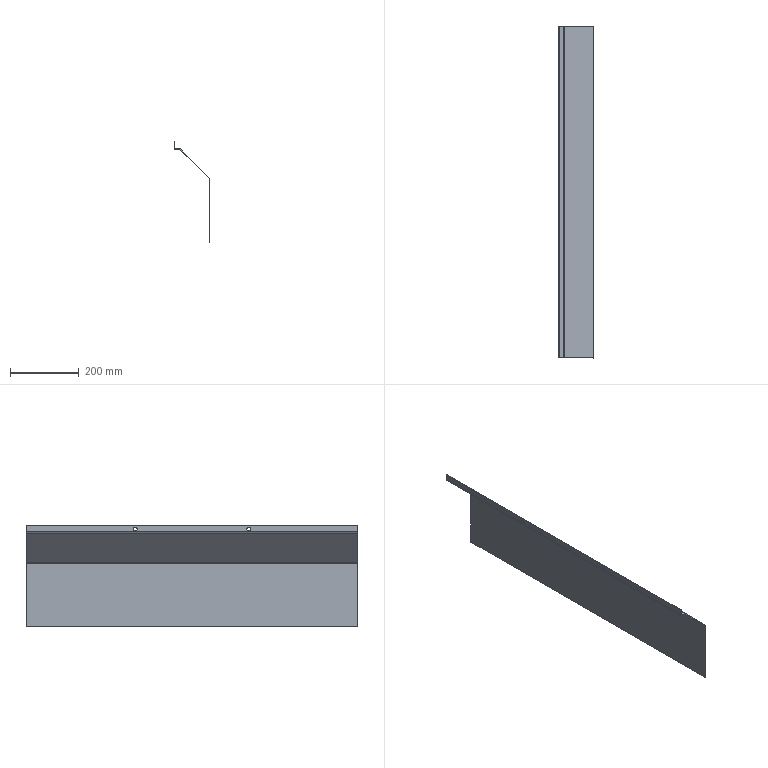Part | STEP file | SYL_0392D6J1SYL0380DJ100-474592 | 1 solid | 38 faces | box 104 x 964 x 292 mm | volume 494830 mm3 | plane 28 | cylinder 10 | commonest cylinder face diameters 8 x4 4 x3 7 x3
STEP:
#1=CARTESIAN_POINT('',(0.,163.,6.));
#2=VERTEX_POINT('',#1);
#3=CARTESIAN_POINT('',(-1.5,163.,6.));
#4=VERTEX_POINT('',#3);
#5=CARTESIAN_POINT('',(-1.5,163.,6.));
#6=DIRECTION('',(-1.,0.,0.));
#7=VECTOR('',#6,1000.);
#8=LINE('',#5,#7);
#9=EDGE_CURVE('',#2,#4,#8,.T.);
#10=ORIENTED_EDGE('',*,*,#9,.F.);
#11=CARTESIAN_POINT('',(0.,167.,6.));
#12=VERTEX_POINT('',#11);
#13=CARTESIAN_POINT('',(0.,-482.,6.));
#14=DIRECTION('',(0.,1.,0.));
#15=VECTOR('',#14,1000.);
#16=LINE('',#13,#15);
#17=EDGE_CURVE('',#2,#12,#16,.T.);
#18=ORIENTED_EDGE('',*,*,#17,.T.);
#19=CARTESIAN_POINT('',(-1.5,167.,6.));
#20=VERTEX_POINT('',#19);
#21=CARTESIAN_POINT('',(-1.5,167.,6.));
#22=DIRECTION('',(-1.,0.,0.));
#23=VECTOR('',#22,1000.);
#24=LINE('',#21,#23);
#25=EDGE_CURVE('',#12,#20,#24,.T.);
#26=ORIENTED_EDGE('',*,*,#25,.T.);
#27=CARTESIAN_POINT('',(-1.5,163.,6.));
#28=DIRECTION('',(0.,1.,0.));
#29=VECTOR('',#28,1000.);
#30=LINE('',#27,#29);
#31=EDGE_CURVE('',#4,#20,#30,.T.);
#32=ORIENTED_EDGE('',*,*,#31,.F.);
#33=EDGE_LOOP('',(#10,#18,#26,#32));
#34=FACE_OUTER_BOUND('',#33,.T.);
#35=CARTESIAN_POINT('',(-1.5,163.,6.));
#36=DIRECTION('',(0.,0.,-1.));
#37=DIRECTION('',(0.,1.,0.));
#38=AXIS2_PLACEMENT_3D('',#35,#36,#37);
#39=PLANE('',#38);
#40=ADVANCED_FACE('',(#34),#39,.F.);
#41=ORIENTED_EDGE('',*,*,#25,.F.);
#42=CARTESIAN_POINT('',(0.,167.,14.));
#43=VERTEX_POINT('',#42);
#44=CARTESIAN_POINT('',(0.,167.,10.));
#45=DIRECTION('',(1.,0.,0.));
#46=DIRECTION('',(0.,0.,-1.));
#47=AXIS2_PLACEMENT_3D('',#44,#45,#46);
#48=CIRCLE('',#47,4.);
#49=EDGE_CURVE('',#12,#43,#48,.T.);
#50=ORIENTED_EDGE('',*,*,#49,.T.);
#51=CARTESIAN_POINT('',(-1.5,167.,14.));
#52=VERTEX_POINT('',#51);
#53=CARTESIAN_POINT('',(-1.5,167.,14.));
#54=DIRECTION('',(-1.,0.,0.));
#55=VECTOR('',#54,1000.);
#56=LINE('',#53,#55);
#57=EDGE_CURVE('',#43,#52,#56,.T.);
#58=ORIENTED_EDGE('',*,*,#57,.T.);
#59=CARTESIAN_POINT('',(-1.5,167.,10.));
#60=DIRECTION('',(1.,0.,0.));
#61=DIRECTION('',(0.,0.,-1.));
#62=AXIS2_PLACEMENT_3D('',#59,#60,#61);
#63=CIRCLE('',#62,4.);
#64=EDGE_CURVE('',#20,#52,#63,.T.);
#65=ORIENTED_EDGE('',*,*,#64,.F.);
#66=EDGE_LOOP('',(#41,#50,#58,#65));
#67=FACE_OUTER_BOUND('',#66,.T.);
#68=CARTESIAN_POINT('',(-1.5,167.,10.));
#69=DIRECTION('',(1.,0.,0.));
#70=DIRECTION('',(0.,0.,-1.));
#71=AXIS2_PLACEMENT_3D('',#68,#69,#70);
#72=CYLINDRICAL_SURFACE('',#71,4.);
#73=ADVANCED_FACE('',(#67),#72,.F.);
#74=ORIENTED_EDGE('',*,*,#57,.F.);
#75=CARTESIAN_POINT('',(0.,163.,14.));
#76=VERTEX_POINT('',#75);
#77=CARTESIAN_POINT('',(0.,-482.,14.));
#78=DIRECTION('',(0.,-1.,0.));
#79=VECTOR('',#78,1000.);
#80=LINE('',#77,#79);
#81=EDGE_CURVE('',#43,#76,#80,.T.);
#82=ORIENTED_EDGE('',*,*,#81,.T.);
#83=CARTESIAN_POINT('',(-1.5,163.,14.));
#84=VERTEX_POINT('',#83);
#85=CARTESIAN_POINT('',(-1.5,163.,14.));
#86=DIRECTION('',(-1.,0.,0.));
#87=VECTOR('',#86,1000.);
#88=LINE('',#85,#87);
#89=EDGE_CURVE('',#76,#84,#88,.T.);
#90=ORIENTED_EDGE('',*,*,#89,.T.);
#91=CARTESIAN_POINT('',(-1.5,167.,14.));
#92=DIRECTION('',(0.,-1.,0.));
#93=VECTOR('',#92,1000.);
#94=LINE('',#91,#93);
#95=EDGE_CURVE('',#52,#84,#94,.T.);
#96=ORIENTED_EDGE('',*,*,#95,.F.);
#97=EDGE_LOOP('',(#74,#82,#90,#96));
#98=FACE_OUTER_BOUND('',#97,.T.);
#99=CARTESIAN_POINT('',(-1.5,167.,14.));
#100=DIRECTION('',(0.,0.,1.));
#101=DIRECTION('',(0.,-1.,0.));
#102=AXIS2_PLACEMENT_3D('',#99,#100,#101);
#103=PLANE('',#102);
#104=ADVANCED_FACE('',(#98),#103,.F.);
#105=CARTESIAN_POINT('',(0.,-163.,6.));
#106=VERTEX_POINT('',#105);
#107=CARTESIAN_POINT('',(-1.5,-163.,6.));
#108=VERTEX_POINT('',#107);
#109=CARTESIAN_POINT('',(-1.5,-163.,6.));
#110=DIRECTION('',(-1.,0.,0.));
#111=VECTOR('',#110,1000.);
#112=LINE('',#109,#111);
#113=EDGE_CURVE('',#106,#108,#112,.T.);
#114=ORIENTED_EDGE('',*,*,#113,.F.);
#115=CARTESIAN_POINT('',(0.,-163.,14.));
#116=VERTEX_POINT('',#115);
#117=CARTESIAN_POINT('',(0.,-163.,10.));
#118=DIRECTION('',(1.,0.,0.));
#119=DIRECTION('',(0.,0.,-1.));
#120=AXIS2_PLACEMENT_3D('',#117,#118,#119);
#121=CIRCLE('',#120,4.);
#122=EDGE_CURVE('',#106,#116,#121,.T.);
#123=ORIENTED_EDGE('',*,*,#122,.T.);
#124=CARTESIAN_POINT('',(-1.5,-163.,14.));
#125=VERTEX_POINT('',#124);
#126=CARTESIAN_POINT('',(-1.5,-163.,14.));
#127=DIRECTION('',(-1.,0.,0.));
#128=VECTOR('',#127,1000.);
#129=LINE('',#126,#128);
#130=EDGE_CURVE('',#116,#125,#129,.T.);
#131=ORIENTED_EDGE('',*,*,#130,.T.);
#132=CARTESIAN_POINT('',(-1.5,-163.,10.));
#133=DIRECTION('',(1.,0.,0.));
#134=DIRECTION('',(0.,0.,-1.));
#135=AXIS2_PLACEMENT_3D('',#132,#133,#134);
#136=CIRCLE('',#135,4.);
#137=EDGE_CURVE('',#108,#125,#136,.T.);
#138=ORIENTED_EDGE('',*,*,#137,.F.);
#139=EDGE_LOOP('',(#114,#123,#131,#138));
#140=FACE_OUTER_BOUND('',#139,.T.);
#141=CARTESIAN_POINT('',(-1.5,-163.,10.));
#142=DIRECTION('',(1.,0.,0.));
#143=DIRECTION('',(0.,0.,-1.));
#144=AXIS2_PLACEMENT_3D('',#141,#142,#143);
#145=CYLINDRICAL_SURFACE('',#144,4.);
#146=ADVANCED_FACE('',(#140),#145,.F.);
#147=ORIENTED_EDGE('',*,*,#130,.F.);
#148=CARTESIAN_POINT('',(0.,-167.,14.));
#149=VERTEX_POINT('',#148);
#150=CARTESIAN_POINT('',(0.,-482.,14.));
#151=DIRECTION('',(0.,-1.,0.));
#152=VECTOR('',#151,1000.);
#153=LINE('',#150,#152);
#154=EDGE_CURVE('',#116,#149,#153,.T.);
#155=ORIENTED_EDGE('',*,*,#154,.T.);
#156=CARTESIAN_POINT('',(-1.5,-167.,14.));
#157=VERTEX_POINT('',#156);
#158=CARTESIAN_POINT('',(-1.5,-167.,14.));
#159=DIRECTION('',(-1.,0.,0.));
#160=VECTOR('',#159,1000.);
#161=LINE('',#158,#160);
#162=EDGE_CURVE('',#149,#157,#161,.T.);
#163=ORIENTED_EDGE('',*,*,#162,.T.);
#164=CARTESIAN_POINT('',(-1.5,-163.,14.));
#165=DIRECTION('',(0.,-1.,0.));
#166=VECTOR('',#165,1000.);
#167=LINE('',#164,#166);
#168=EDGE_CURVE('',#125,#157,#167,.T.);
#169=ORIENTED_EDGE('',*,*,#168,.F.);
#170=EDGE_LOOP('',(#147,#155,#163,#169));
#171=FACE_OUTER_BOUND('',#170,.T.);
#172=CARTESIAN_POINT('',(-1.5,-163.,14.));
#173=DIRECTION('',(0.,0.,1.));
#174=DIRECTION('',(0.,-1.,0.));
#175=AXIS2_PLACEMENT_3D('',#172,#173,#174);
#176=PLANE('',#175);
#177=ADVANCED_FACE('',(#171),#176,.F.);
#178=ORIENTED_EDGE('',*,*,#162,.F.);
#179=CARTESIAN_POINT('',(0.,-167.,6.));
#180=VERTEX_POINT('',#179);
#181=CARTESIAN_POINT('',(0.,-167.,10.));
#182=DIRECTION('',(1.,0.,0.));
#183=DIRECTION('',(0.,0.,-1.));
#184=AXIS2_PLACEMENT_3D('',#181,#182,#183);
#185=CIRCLE('',#184,4.);
#186=EDGE_CURVE('',#149,#180,#185,.T.);
#187=ORIENTED_EDGE('',*,*,#186,.T.);
#188=CARTESIAN_POINT('',(-1.5,-167.,6.));
#189=VERTEX_POINT('',#188);
#190=CARTESIAN_POINT('',(-1.5,-167.,6.));
#191=DIRECTION('',(-1.,0.,0.));
#192=VECTOR('',#191,1000.);
#193=LINE('',#190,#192);
#194=EDGE_CURVE('',#180,#189,#193,.T.);
#195=ORIENTED_EDGE('',*,*,#194,.T.);
#196=CARTESIAN_POINT('',(-1.5,-167.,10.));
#197=DIRECTION('',(1.,0.,0.));
#198=DIRECTION('',(0.,0.,1.));
#199=AXIS2_PLACEMENT_3D('',#196,#197,#198);
#200=CIRCLE('',#199,4.);
#201=EDGE_CURVE('',#157,#189,#200,.T.);
#202=ORIENTED_EDGE('',*,*,#201,.F.);
#203=EDGE_LOOP('',(#178,#187,#195,#202));
#204=FACE_OUTER_BOUND('',#203,.T.);
#205=CARTESIAN_POINT('',(-1.5,-167.,10.));
#206=DIRECTION('',(1.,0.,0.));
#207=DIRECTION('',(0.,0.,-1.));
#208=AXIS2_PLACEMENT_3D('',#205,#206,#207);
#209=CYLINDRICAL_SURFACE('',#208,4.);
#210=ADVANCED_FACE('',(#204),#209,.F.);
#211=CARTESIAN_POINT('',(0.,-482.,20.));
#212=VERTEX_POINT('',#211);
#213=CARTESIAN_POINT('',(-1.5,-482.,20.));
#214=VERTEX_POINT('',#213);
#215=CARTESIAN_POINT('',(-1.5,-482.,20.));
#216=DIRECTION('',(-1.,0.,0.));
#217=VECTOR('',#216,1000.);
#218=LINE('',#215,#217);
#219=EDGE_CURVE('',#212,#214,#218,.T.);
#220=ORIENTED_EDGE('',*,*,#219,.F.);
#221=CARTESIAN_POINT('',(0.,482.,20.));
#222=VERTEX_POINT('',#221);
#223=CARTESIAN_POINT('',(0.,-482.,20.));
#224=DIRECTION('',(0.,-1.,0.));
#225=VECTOR('',#224,1000.);
#226=LINE('',#223,#225);
#227=EDGE_CURVE('',#222,#212,#226,.T.);
#228=ORIENTED_EDGE('',*,*,#227,.F.);
#229=CARTESIAN_POINT('',(-1.5,482.,20.));
#230=VERTEX_POINT('',#229);
#231=CARTESIAN_POINT('',(-1.5,482.,20.));
#232=DIRECTION('',(-1.,0.,0.));
#233=VECTOR('',#232,1000.);
#234=LINE('',#231,#233);
#235=EDGE_CURVE('',#222,#230,#234,.T.);
#236=ORIENTED_EDGE('',*,*,#235,.T.);
#237=CARTESIAN_POINT('',(-1.5,482.,20.));
#238=DIRECTION('',(0.,-1.,0.));
#239=VECTOR('',#238,1000.);
#240=LINE('',#237,#239);
#241=EDGE_CURVE('',#230,#214,#240,.T.);
#242=ORIENTED_EDGE('',*,*,#241,.T.);
#243=EDGE_LOOP('',(#220,#228,#236,#242));
#244=FACE_OUTER_BOUND('',#243,.T.);
#245=CARTESIAN_POINT('',(-1.5,482.,20.));
#246=DIRECTION('',(0.,0.,1.));
#247=DIRECTION('',(0.,-1.,0.));
#248=AXIS2_PLACEMENT_3D('',#245,#246,#247);
#249=PLANE('',#248);
#250=ADVANCED_FACE('',(#244),#249,.T.);
#251=ORIENTED_EDGE('',*,*,#235,.F.);
#252=CARTESIAN_POINT('',(0.,482.,2.));
#253=VERTEX_POINT('',#252);
#254=CARTESIAN_POINT('',(0.,482.,20.));
#255=DIRECTION('',(0.,0.,1.));
#256=VECTOR('',#255,1000.);
#257=LINE('',#254,#256);
#258=EDGE_CURVE('',#253,#222,#257,.T.);
#259=ORIENTED_EDGE('',*,*,#258,.F.);
#260=CARTESIAN_POINT('',(-1.5,482.,2.));
#261=VERTEX_POINT('',#260);
#262=CARTESIAN_POINT('',(-1.5,482.,2.));
#263=DIRECTION('',(-1.,0.,0.));
#264=VECTOR('',#263,1000.);
#265=LINE('',#262,#264);
#266=EDGE_CURVE('',#253,#261,#265,.T.);
#267=ORIENTED_EDGE('',*,*,#266,.T.);
#268=CARTESIAN_POINT('',(-1.5,482.,2.));
#269=DIRECTION('',(0.,0.,1.));
#270=VECTOR('',#269,1000.);
#271=LINE('',#268,#270);
#272=EDGE_CURVE('',#261,#230,#271,.T.);
#273=ORIENTED_EDGE('',*,*,#272,.T.);
#274=EDGE_LOOP('',(#251,#259,#267,#273));
#275=FACE_OUTER_BOUND('',#274,.T.);
#276=CARTESIAN_POINT('',(-1.5,482.,2.));
#277=DIRECTION('',(0.,1.,0.));
#278=DIRECTION('',(0.,0.,1.));
#279=AXIS2_PLACEMENT_3D('',#276,#277,#278);
#280=PLANE('',#279);
#281=ADVANCED_FACE('',(#275),#280,.T.);
#282=ORIENTED_EDGE('',*,*,#266,.F.);
#283=CARTESIAN_POINT('',(2.,482.,0.));
#284=VERTEX_POINT('',#283);
#285=CARTESIAN_POINT('',(2.,482.,2.));
#286=DIRECTION('',(0.,1.,0.));
#287=DIRECTION('',(0.,0.,1.));
#288=AXIS2_PLACEMENT_3D('',#285,#286,#287);
#289=CIRCLE('',#288,2.);
#290=EDGE_CURVE('',#284,#253,#289,.T.);
#291=ORIENTED_EDGE('',*,*,#290,.F.);
#292=CARTESIAN_POINT('',(2.,482.,-1.5));
#293=VERTEX_POINT('',#292);
#294=CARTESIAN_POINT('',(2.,482.,-1.5));
#295=DIRECTION('',(0.,0.,-1.));
#296=VECTOR('',#295,1000.);
#297=LINE('',#294,#296);
#298=EDGE_CURVE('',#284,#293,#297,.T.);
#299=ORIENTED_EDGE('',*,*,#298,.T.);
#300=CARTESIAN_POINT('',(2.,482.,2.));
#301=DIRECTION('',(0.,1.,0.));
#302=DIRECTION('',(0.,0.,-1.));
#303=AXIS2_PLACEMENT_3D('',#300,#301,#302);
#304=CIRCLE('',#303,3.5);
#305=EDGE_CURVE('',#293,#261,#304,.T.);
#306=ORIENTED_EDGE('',*,*,#305,.T.);
#307=EDGE_LOOP('',(#282,#291,#299,#306));
#308=FACE_OUTER_BOUND('',#307,.T.);
#309=CARTESIAN_POINT('',(2.,482.,2.));
#310=DIRECTION('',(0.,-1.,0.));
#311=DIRECTION('',(0.,0.,-1.));
#312=AXIS2_PLACEMENT_3D('',#309,#310,#311);
#313=PLANE('',#312);
#314=ADVANCED_FACE('',(#308),#313,.F.);
#315=ORIENTED_EDGE('',*,*,#298,.F.);
#316=CARTESIAN_POINT('',(14.05,482.,0.));
#317=VERTEX_POINT('',#316);
#318=CARTESIAN_POINT('',(0.,482.,0.));
#319=DIRECTION('',(-1.,0.,0.));
#320=VECTOR('',#319,1000.);
#321=LINE('',#318,#320);
#322=EDGE_CURVE('',#317,#284,#321,.T.);
#323=ORIENTED_EDGE('',*,*,#322,.F.);
#324=CARTESIAN_POINT('',(14.05,482.,-1.5));
#325=VERTEX_POINT('',#324);
#326=CARTESIAN_POINT('',(14.05,482.,-1.5));
#327=DIRECTION('',(0.,0.,-1.));
#328=VECTOR('',#327,1000.);
#329=LINE('',#326,#328);
#330=EDGE_CURVE('',#317,#325,#329,.T.);
#331=ORIENTED_EDGE('',*,*,#330,.T.);
#332=CARTESIAN_POINT('',(14.05,482.,-1.5));
#333=DIRECTION('',(-1.,0.,0.));
#334=VECTOR('',#333,1000.);
#335=LINE('',#332,#334);
#336=EDGE_CURVE('',#325,#293,#335,.T.);
#337=ORIENTED_EDGE('',*,*,#336,.T.);
#338=EDGE_LOOP('',(#315,#323,#331,#337));
#339=FACE_OUTER_BOUND('',#338,.T.);
#340=CARTESIAN_POINT('',(14.05,482.,-1.5));
#341=DIRECTION('',(0.,1.,0.));
#342=DIRECTION('',(-1.,0.,0.));
#343=AXIS2_PLACEMENT_3D('',#340,#341,#342);
#344=PLANE('',#343);
#345=ADVANCED_FACE('',(#339),#344,.T.);
#346=ORIENTED_EDGE('',*,*,#330,.F.);
#347=CARTESIAN_POINT('',(16.525,482.,-1.025));
#348=VERTEX_POINT('',#347);
#349=CARTESIAN_POINT('',(14.05,482.,-3.5));
#350=DIRECTION('',(0.,-1.,0.));
#351=DIRECTION('',(0.,0.,-1.));
#352=AXIS2_PLACEMENT_3D('',#349,#350,#351);
#353=CIRCLE('',#352,3.5);
#354=EDGE_CURVE('',#348,#317,#353,.T.);
#355=ORIENTED_EDGE('',*,*,#354,.F.);
#356=CARTESIAN_POINT('',(15.464,482.,-2.086));
#357=VERTEX_POINT('',#356);
#358=CARTESIAN_POINT('',(15.464,482.,-2.086));
#359=DIRECTION('',(-0.7071,0.,-0.7071));
#360=VECTOR('',#359,1000.);
#361=LINE('',#358,#360);
#362=EDGE_CURVE('',#348,#357,#361,.T.);
#363=ORIENTED_EDGE('',*,*,#362,.T.);
#364=CARTESIAN_POINT('',(14.05,482.,-3.5));
#365=DIRECTION('',(0.,-1.,0.));
#366=DIRECTION('',(0.7071,0.,0.7071));
#367=AXIS2_PLACEMENT_3D('',#364,#365,#366);
#368=CIRCLE('',#367,2.);
#369=EDGE_CURVE('',#357,#325,#368,.T.);
#370=ORIENTED_EDGE('',*,*,#369,.T.);
#371=EDGE_LOOP('',(#346,#355,#363,#370));
#372=FACE_OUTER_BOUND('',#371,.T.);
#373=CARTESIAN_POINT('',(14.05,482.,-3.5));
#374=DIRECTION('',(0.,1.,0.));
#375=DIRECTION('',(0.,0.,1.));
#376=AXIS2_PLACEMENT_3D('',#373,#374,#375);
#377=PLANE('',#376);
#378=ADVANCED_FACE('',(#372),#377,.T.);
#379=ORIENTED_EDGE('',*,*,#362,.F.);
#380=CARTESIAN_POINT('',(101.475,482.,-85.975));
#381=VERTEX_POINT('',#380);
#382=CARTESIAN_POINT('',(15.5,482.,0.));
#383=DIRECTION('',(-0.7071,0.,0.7071));
#384=VECTOR('',#383,1000.);
#385=LINE('',#382,#384);
#386=EDGE_CURVE('',#381,#348,#385,.T.);
#387=ORIENTED_EDGE('',*,*,#386,.F.);
#388=CARTESIAN_POINT('',(100.414,482.,-87.036));
#389=VERTEX_POINT('',#388);
#390=CARTESIAN_POINT('',(100.414,482.,-87.036));
#391=DIRECTION('',(-0.7071,0.,-0.7071));
#392=VECTOR('',#391,1000.);
#393=LINE('',#390,#392);
#394=EDGE_CURVE('',#381,#389,#393,.T.);
#395=ORIENTED_EDGE('',*,*,#394,.T.);
#396=CARTESIAN_POINT('',(100.414,482.,-87.036));
#397=DIRECTION('',(-0.7071,0.,0.7071));
#398=VECTOR('',#397,1000.);
#399=LINE('',#396,#398);
#400=EDGE_CURVE('',#389,#357,#399,.T.);
#401=ORIENTED_EDGE('',*,*,#400,.T.);
#402=EDGE_LOOP('',(#379,#387,#395,#401));
#403=FACE_OUTER_BOUND('',#402,.T.);
#404=CARTESIAN_POINT('',(100.414,482.,-87.036));
#405=DIRECTION('',(0.,1.,0.));
#406=DIRECTION('',(-0.7071,0.,0.7071));
#407=AXIS2_PLACEMENT_3D('',#404,#405,#406);
#408=PLANE('',#407);
#409=ADVANCED_FACE('',(#403),#408,.T.);
#410=ORIENTED_EDGE('',*,*,#394,.F.);
#411=CARTESIAN_POINT('',(102.5,482.,-88.45));
#412=VERTEX_POINT('',#411);
#413=CARTESIAN_POINT('',(99.,482.,-88.45));
#414=DIRECTION('',(0.,-1.,0.));
#415=DIRECTION('',(0.,0.,-1.));
#416=AXIS2_PLACEMENT_3D('',#413,#414,#415);
#417=CIRCLE('',#416,3.5);
#418=EDGE_CURVE('',#412,#381,#417,.T.);
#419=ORIENTED_EDGE('',*,*,#418,.F.);
#420=CARTESIAN_POINT('',(101.,482.,-88.45));
#421=VERTEX_POINT('',#420);
#422=CARTESIAN_POINT('',(101.,482.,-88.45));
#423=DIRECTION('',(-1.,0.,0.));
#424=VECTOR('',#423,1000.);
#425=LINE('',#422,#424);
#426=EDGE_CURVE('',#412,#421,#425,.T.);
#427=ORIENTED_EDGE('',*,*,#426,.T.);
#428=CARTESIAN_POINT('',(99.,482.,-88.45));
#429=DIRECTION('',(0.,-1.,0.));
#430=DIRECTION('',(1.,0.,0.));
#431=AXIS2_PLACEMENT_3D('',#428,#429,#430);
#432=CIRCLE('',#431,2.);
#433=EDGE_CURVE('',#421,#389,#432,.T.);
#434=ORIENTED_EDGE('',*,*,#433,.T.);
#435=EDGE_LOOP('',(#410,#419,#427,#434));
#436=FACE_OUTER_BOUND('',#435,.T.);
#437=CARTESIAN_POINT('',(99.,482.,-88.45));
#438=DIRECTION('',(0.,1.,0.));
#439=DIRECTION('',(0.,0.,1.));
#440=AXIS2_PLACEMENT_3D('',#437,#438,#439);
#441=PLANE('',#440);
#442=ADVANCED_FACE('',(#436),#441,.T.);
#443=ORIENTED_EDGE('',*,*,#426,.F.);
#444=CARTESIAN_POINT('',(102.5,482.,-272.));
#445=VERTEX_POINT('',#444);
#446=CARTESIAN_POINT('',(102.5,482.,-87.));
#447=DIRECTION('',(0.,0.,1.));
#448=VECTOR('',#447,1000.);
#449=LINE('',#446,#448);
#450=EDGE_CURVE('',#445,#412,#449,.T.);
#451=ORIENTED_EDGE('',*,*,#450,.F.);
#452=CARTESIAN_POINT('',(101.,482.,-272.));
#453=VERTEX_POINT('',#452);
#454=CARTESIAN_POINT('',(101.,482.,-272.));
#455=DIRECTION('',(-1.,0.,0.));
#456=VECTOR('',#455,1000.);
#457=LINE('',#454,#456);
#458=EDGE_CURVE('',#445,#453,#457,.T.);
#459=ORIENTED_EDGE('',*,*,#458,.T.);
#460=CARTESIAN_POINT('',(101.,482.,-272.));
#461=DIRECTION('',(0.,0.,1.));
#462=VECTOR('',#461,1000.);
#463=LINE('',#460,#462);
#464=EDGE_CURVE('',#453,#421,#463,.T.);
#465=ORIENTED_EDGE('',*,*,#464,.T.);
#466=EDGE_LOOP('',(#443,#451,#459,#465));
#467=FACE_OUTER_BOUND('',#466,.T.);
#468=CARTESIAN_POINT('',(101.,482.,-272.));
#469=DIRECTION('',(0.,1.,0.));
#470=DIRECTION('',(0.,0.,1.));
#471=AXIS2_PLACEMENT_3D('',#468,#469,#470);
#472=PLANE('',#471);
#473=ADVANCED_FACE('',(#467),#472,.T.);
#474=ORIENTED_EDGE('',*,*,#458,.F.);
#475=CARTESIAN_POINT('',(102.5,-482.,-272.));
#476=VERTEX_POINT('',#475);
#477=CARTESIAN_POINT('',(102.5,-482.,-272.));
#478=DIRECTION('',(0.,-1.,0.));
#479=VECTOR('',#478,1000.);
#480=LINE('',#477,#479);
#481=EDGE_CURVE('',#445,#476,#480,.T.);
#482=ORIENTED_EDGE('',*,*,#481,.T.);
#483=CARTESIAN_POINT('',(101.,-482.,-272.));
#484=VERTEX_POINT('',#483);
#485=CARTESIAN_POINT('',(101.,-482.,-272.));
#486=DIRECTION('',(-1.,0.,0.));
#487=VECTOR('',#486,1000.);
#488=LINE('',#485,#487);
#489=EDGE_CURVE('',#476,#484,#488,.T.);
#490=ORIENTED_EDGE('',*,*,#489,.T.);
#491=CARTESIAN_POINT('',(101.,482.,-272.));
#492=DIRECTION('',(0.,-1.,0.));
#493=VECTOR('',#492,1000.);
#494=LINE('',#491,#493);
#495=EDGE_CURVE('',#453,#484,#494,.T.);
#496=ORIENTED_EDGE('',*,*,#495,.F.);
#497=EDGE_LOOP('',(#474,#482,#490,#496));
#498=FACE_OUTER_BOUND('',#497,.T.);
#499=CARTESIAN_POINT('',(101.,482.,-272.));
#500=DIRECTION('',(0.,0.,1.));
#501=DIRECTION('',(0.,-1.,0.));
#502=AXIS2_PLACEMENT_3D('',#499,#500,#501);
#503=PLANE('',#502);
#504=ADVANCED_FACE('',(#498),#503,.F.);
#505=ORIENTED_EDGE('',*,*,#489,.F.);
#506=CARTESIAN_POINT('',(102.5,-482.,-88.45));
#507=VERTEX_POINT('',#506);
#508=CARTESIAN_POINT('',(102.5,-482.,-87.));
#509=DIRECTION('',(0.,0.,1.));
#510=VECTOR('',#509,1000.);
#511=LINE('',#508,#510);
#512=EDGE_CURVE('',#476,#507,#511,.T.);
#513=ORIENTED_EDGE('',*,*,#512,.T.);
#514=CARTESIAN_POINT('',(101.,-482.,-88.45));
#515=VERTEX_POINT('',#514);
#516=CARTESIAN_POINT('',(101.,-482.,-88.45));
#517=DIRECTION('',(-1.,0.,0.));
#518=VECTOR('',#517,1000.);
#519=LINE('',#516,#518);
#520=EDGE_CURVE('',#507,#515,#519,.T.);
#521=ORIENTED_EDGE('',*,*,#520,.T.);
#522=CARTESIAN_POINT('',(101.,-482.,-272.));
#523=DIRECTION('',(0.,0.,1.));
#524=VECTOR('',#523,1000.);
#525=LINE('',#522,#524);
#526=EDGE_CURVE('',#484,#515,#525,.T.);
#527=ORIENTED_EDGE('',*,*,#526,.F.);
#528=EDGE_LOOP('',(#505,#513,#521,#527));
#529=FACE_OUTER_BOUND('',#528,.T.);
#530=CARTESIAN_POINT('',(101.,-482.,-272.));
#531=DIRECTION('',(0.,1.,0.));
#532=DIRECTION('',(0.,0.,1.));
#533=AXIS2_PLACEMENT_3D('',#530,#531,#532);
#534=PLANE('',#533);
#535=ADVANCED_FACE('',(#529),#534,.F.);
#536=ORIENTED_EDGE('',*,*,#520,.F.);
#537=CARTESIAN_POINT('',(101.475,-482.,-85.975));
#538=VERTEX_POINT('',#537);
#539=CARTESIAN_POINT('',(99.,-482.,-88.45));
#540=DIRECTION('',(0.,1.,0.));
#541=DIRECTION('',(0.,0.,-1.));
#542=AXIS2_PLACEMENT_3D('',#539,#540,#541);
#543=CIRCLE('',#542,3.5);
#544=EDGE_CURVE('',#538,#507,#543,.T.);
#545=ORIENTED_EDGE('',*,*,#544,.F.);
#546=CARTESIAN_POINT('',(100.414,-482.,-87.036));
#547=VERTEX_POINT('',#546);
#548=CARTESIAN_POINT('',(100.414,-482.,-87.036));
#549=DIRECTION('',(-0.7071,0.,-0.7071));
#550=VECTOR('',#549,1000.);
#551=LINE('',#548,#550);
#552=EDGE_CURVE('',#538,#547,#551,.T.);
#553=ORIENTED_EDGE('',*,*,#552,.T.);
#554=CARTESIAN_POINT('',(99.,-482.,-88.45));
#555=DIRECTION('',(0.,1.,0.));
#556=DIRECTION('',(0.7071,0.,0.7071));
#557=AXIS2_PLACEMENT_3D('',#554,#555,#556);
#558=CIRCLE('',#557,2.);
#559=EDGE_CURVE('',#547,#515,#558,.T.);
#560=ORIENTED_EDGE('',*,*,#559,.T.);
#561=EDGE_LOOP('',(#536,#545,#553,#560));
#562=FACE_OUTER_BOUND('',#561,.T.);
#563=CARTESIAN_POINT('',(99.,-482.,-88.45));
#564=DIRECTION('',(0.,-1.,0.));
#565=DIRECTION('',(0.,0.,-1.));
#566=AXIS2_PLACEMENT_3D('',#563,#564,#565);
#567=PLANE('',#566);
#568=ADVANCED_FACE('',(#562),#567,.T.);
#569=ORIENTED_EDGE('',*,*,#552,.F.);
#570=CARTESIAN_POINT('',(16.525,-482.,-1.025));
#571=VERTEX_POINT('',#570);
#572=CARTESIAN_POINT('',(15.5,-482.,0.));
#573=DIRECTION('',(0.7071,0.,-0.7071));
#574=VECTOR('',#573,1000.);
#575=LINE('',#572,#574);
#576=EDGE_CURVE('',#571,#538,#575,.T.);
#577=ORIENTED_EDGE('',*,*,#576,.F.);
#578=CARTESIAN_POINT('',(15.464,-482.,-2.086));
#579=VERTEX_POINT('',#578);
#580=CARTESIAN_POINT('',(15.464,-482.,-2.086));
#581=DIRECTION('',(-0.7071,0.,-0.7071));
#582=VECTOR('',#581,1000.);
#583=LINE('',#580,#582);
#584=EDGE_CURVE('',#571,#579,#583,.T.);
#585=ORIENTED_EDGE('',*,*,#584,.T.);
#586=CARTESIAN_POINT('',(15.464,-482.,-2.086));
#587=DIRECTION('',(0.7071,0.,-0.7071));
#588=VECTOR('',#587,1000.);
#589=LINE('',#586,#588);
#590=EDGE_CURVE('',#579,#547,#589,.T.);
#591=ORIENTED_EDGE('',*,*,#590,.T.);
#592=EDGE_LOOP('',(#569,#577,#585,#591));
#593=FACE_OUTER_BOUND('',#592,.T.);
#594=CARTESIAN_POINT('',(15.464,-482.,-2.086));
#595=DIRECTION('',(0.,-1.,0.));
#596=DIRECTION('',(0.7071,0.,-0.7071));
#597=AXIS2_PLACEMENT_3D('',#594,#595,#596);
#598=PLANE('',#597);
#599=ADVANCED_FACE('',(#593),#598,.T.);
#600=ORIENTED_EDGE('',*,*,#584,.F.);
#601=CARTESIAN_POINT('',(14.05,-482.,0.));
#602=VERTEX_POINT('',#601);
#603=CARTESIAN_POINT('',(14.05,-482.,-3.5));
#604=DIRECTION('',(0.,1.,0.));
#605=DIRECTION('',(0.,0.,-1.));
#606=AXIS2_PLACEMENT_3D('',#603,#604,#605);
#607=CIRCLE('',#606,3.5);
#608=EDGE_CURVE('',#602,#571,#607,.T.);
#609=ORIENTED_EDGE('',*,*,#608,.F.);
#610=CARTESIAN_POINT('',(14.05,-482.,-1.5));
#611=VERTEX_POINT('',#610);
#612=CARTESIAN_POINT('',(14.05,-482.,-1.5));
#613=DIRECTION('',(0.,0.,-1.));
#614=VECTOR('',#613,1000.);
#615=LINE('',#612,#614);
#616=EDGE_CURVE('',#602,#611,#615,.T.);
#617=ORIENTED_EDGE('',*,*,#616,.T.);
#618=CARTESIAN_POINT('',(14.05,-482.,-3.5));
#619=DIRECTION('',(0.,1.,0.));
#620=DIRECTION('',(0.,0.,1.));
#621=AXIS2_PLACEMENT_3D('',#618,#619,#620);
#622=CIRCLE('',#621,2.);
#623=EDGE_CURVE('',#611,#579,#622,.T.);
#624=ORIENTED_EDGE('',*,*,#623,.T.);
#625=EDGE_LOOP('',(#600,#609,#617,#624));
#626=FACE_OUTER_BOUND('',#625,.T.);
#627=CARTESIAN_POINT('',(14.05,-482.,-3.5));
#628=DIRECTION('',(0.,-1.,0.));
#629=DIRECTION('',(0.,0.,-1.));
#630=AXIS2_PLACEMENT_3D('',#627,#628,#629);
#631=PLANE('',#630);
#632=ADVANCED_FACE('',(#626),#631,.T.);
#633=ORIENTED_EDGE('',*,*,#616,.F.);
#634=CARTESIAN_POINT('',(2.,-482.,0.));
#635=VERTEX_POINT('',#634);
#636=CARTESIAN_POINT('',(0.,-482.,0.));
#637=DIRECTION('',(-1.,0.,0.));
#638=VECTOR('',#637,1000.);
#639=LINE('',#636,#638);
#640=EDGE_CURVE('',#602,#635,#639,.T.);
#641=ORIENTED_EDGE('',*,*,#640,.T.);
#642=CARTESIAN_POINT('',(2.,-482.,-1.5));
#643=VERTEX_POINT('',#642);
#644=CARTESIAN_POINT('',(2.,-482.,-1.5));
#645=DIRECTION('',(0.,0.,-1.));
#646=VECTOR('',#645,1000.);
#647=LINE('',#644,#646);
#648=EDGE_CURVE('',#635,#643,#647,.T.);
#649=ORIENTED_EDGE('',*,*,#648,.T.);
#650=CARTESIAN_POINT('',(14.05,-482.,-1.5));
#651=DIRECTION('',(-1.,0.,0.));
#652=VECTOR('',#651,1000.);
#653=LINE('',#650,#652);
#654=EDGE_CURVE('',#611,#643,#653,.T.);
#655=ORIENTED_EDGE('',*,*,#654,.F.);
#656=EDGE_LOOP('',(#633,#641,#649,#655));
#657=FACE_OUTER_BOUND('',#656,.T.);
#658=CARTESIAN_POINT('',(14.05,-482.,-1.5));
#659=DIRECTION('',(0.,1.,0.));
#660=DIRECTION('',(-1.,0.,0.));
#661=AXIS2_PLACEMENT_3D('',#658,#659,#660);
#662=PLANE('',#661);
#663=ADVANCED_FACE('',(#657),#662,.F.);
#664=ORIENTED_EDGE('',*,*,#648,.F.);
#665=CARTESIAN_POINT('',(0.,-482.,2.));
#666=VERTEX_POINT('',#665);
#667=CARTESIAN_POINT('',(2.,-482.,2.));
#668=DIRECTION('',(0.,-1.,0.));
#669=DIRECTION('',(0.,0.,1.));
#670=AXIS2_PLACEMENT_3D('',#667,#668,#669);
#671=CIRCLE('',#670,2.);
#672=EDGE_CURVE('',#666,#635,#671,.T.);
#673=ORIENTED_EDGE('',*,*,#672,.F.);
#674=CARTESIAN_POINT('',(-1.5,-482.,2.));
#675=VERTEX_POINT('',#674);
#676=CARTESIAN_POINT('',(-1.5,-482.,2.));
#677=DIRECTION('',(-1.,0.,0.));
#678=VECTOR('',#677,1000.);
#679=LINE('',#676,#678);
#680=EDGE_CURVE('',#666,#675,#679,.T.);
#681=ORIENTED_EDGE('',*,*,#680,.T.);
#682=CARTESIAN_POINT('',(2.,-482.,2.));
#683=DIRECTION('',(0.,-1.,0.));
#684=DIRECTION('',(-1.,0.,0.));
#685=AXIS2_PLACEMENT_3D('',#682,#683,#684);
#686=CIRCLE('',#685,3.5);
#687=EDGE_CURVE('',#675,#643,#686,.T.);
#688=ORIENTED_EDGE('',*,*,#687,.T.);
#689=EDGE_LOOP('',(#664,#673,#681,#688));
#690=FACE_OUTER_BOUND('',#689,.T.);
#691=CARTESIAN_POINT('',(2.,-482.,2.));
#692=DIRECTION('',(0.,1.,0.));
#693=DIRECTION('',(0.,0.,1.));
#694=AXIS2_PLACEMENT_3D('',#691,#692,#693);
#695=PLANE('',#694);
#696=ADVANCED_FACE('',(#690),#695,.F.);
#697=CARTESIAN_POINT('',(0.,-482.,6.));
#698=DIRECTION('',(0.,1.,0.));
#699=VECTOR('',#698,1000.);
#700=LINE('',#697,#699);
#701=EDGE_CURVE('',#180,#106,#700,.T.);
#702=ORIENTED_EDGE('',*,*,#701,.T.);
#703=ORIENTED_EDGE('',*,*,#113,.T.);
#704=CARTESIAN_POINT('',(-1.5,-167.,6.));
#705=DIRECTION('',(0.,1.,0.));
#706=VECTOR('',#705,1000.);
#707=LINE('',#704,#706);
#708=EDGE_CURVE('',#189,#108,#707,.T.);
#709=ORIENTED_EDGE('',*,*,#708,.F.);
#710=ORIENTED_EDGE('',*,*,#194,.F.);
#711=EDGE_LOOP('',(#702,#703,#709,#710));
#712=FACE_OUTER_BOUND('',#711,.T.);
#713=CARTESIAN_POINT('',(-1.5,-167.,6.));
#714=DIRECTION('',(0.,0.,-1.));
#715=DIRECTION('',(0.,1.,0.));
#716=AXIS2_PLACEMENT_3D('',#713,#714,#715);
#717=PLANE('',#716);
#718=ADVANCED_FACE('',(#712),#717,.F.);
#719=CARTESIAN_POINT('',(0.,163.,10.));
#720=DIRECTION('',(1.,0.,0.));
#721=DIRECTION('',(0.,0.,-1.));
#722=AXIS2_PLACEMENT_3D('',#719,#720,#721);
#723=CIRCLE('',#722,4.);
#724=EDGE_CURVE('',#76,#2,#723,.T.);
#725=ORIENTED_EDGE('',*,*,#724,.T.);
#726=ORIENTED_EDGE('',*,*,#9,.T.);
#727=CARTESIAN_POINT('',(-1.5,163.,10.));
#728=DIRECTION('',(1.,0.,0.));
#729=DIRECTION('',(0.,0.,1.));
#730=AXIS2_PLACEMENT_3D('',#727,#728,#729);
#731=CIRCLE('',#730,4.);
#732=EDGE_CURVE('',#84,#4,#731,.T.);
#733=ORIENTED_EDGE('',*,*,#732,.F.);
#734=ORIENTED_EDGE('',*,*,#89,.F.);
#735=EDGE_LOOP('',(#725,#726,#733,#734));
#736=FACE_OUTER_BOUND('',#735,.T.);
#737=CARTESIAN_POINT('',(-1.5,163.,10.));
#738=DIRECTION('',(1.,0.,0.));
#739=DIRECTION('',(0.,0.,-1.));
#740=AXIS2_PLACEMENT_3D('',#737,#738,#739);
#741=CYLINDRICAL_SURFACE('',#740,4.);
#742=ADVANCED_FACE('',(#736),#741,.F.);
#743=CARTESIAN_POINT('',(0.,-482.,20.));
#744=DIRECTION('',(0.,0.,1.));
#745=VECTOR('',#744,1000.);
#746=LINE('',#743,#745);
#747=EDGE_CURVE('',#666,#212,#746,.T.);
#748=ORIENTED_EDGE('',*,*,#747,.T.);
#749=ORIENTED_EDGE('',*,*,#219,.T.);
#750=CARTESIAN_POINT('',(-1.5,-482.,2.));
#751=DIRECTION('',(0.,0.,1.));
#752=VECTOR('',#751,1000.);
#753=LINE('',#750,#752);
#754=EDGE_CURVE('',#675,#214,#753,.T.);
#755=ORIENTED_EDGE('',*,*,#754,.F.);
#756=ORIENTED_EDGE('',*,*,#680,.F.);
#757=EDGE_LOOP('',(#748,#749,#755,#756));
#758=FACE_OUTER_BOUND('',#757,.T.);
#759=CARTESIAN_POINT('',(-1.5,-482.,2.));
#760=DIRECTION('',(0.,1.,0.));
#761=DIRECTION('',(0.,0.,1.));
#762=AXIS2_PLACEMENT_3D('',#759,#760,#761);
#763=PLANE('',#762);
#764=ADVANCED_FACE('',(#758),#763,.F.);
#765=CARTESIAN_POINT('',(2.,482.,-1.5));
#766=DIRECTION('',(0.,-1.,0.));
#767=VECTOR('',#766,1000.);
#768=LINE('',#765,#767);
#769=EDGE_CURVE('',#293,#643,#768,.T.);
#770=ORIENTED_EDGE('',*,*,#769,.T.);
#771=ORIENTED_EDGE('',*,*,#687,.F.);
#772=CARTESIAN_POINT('',(-1.5,-482.,2.));
#773=DIRECTION('',(0.,1.,0.));
#774=VECTOR('',#773,1000.);
#775=LINE('',#772,#774);
#776=EDGE_CURVE('',#675,#261,#775,.T.);
#777=ORIENTED_EDGE('',*,*,#776,.T.);
#778=ORIENTED_EDGE('',*,*,#305,.F.);
#779=EDGE_LOOP('',(#770,#771,#777,#778));
#780=FACE_OUTER_BOUND('',#779,.T.);
#781=CARTESIAN_POINT('',(2.,-482.,2.));
#782=DIRECTION('',(0.,1.,0.));
#783=DIRECTION('',(0.,0.,1.));
#784=AXIS2_PLACEMENT_3D('',#781,#782,#783);
#785=CYLINDRICAL_SURFACE('',#784,3.5);
#786=ADVANCED_FACE('',(#780),#785,.T.);
#787=ORIENTED_EDGE('',*,*,#201,.T.);
#788=ORIENTED_EDGE('',*,*,#708,.T.);
#789=ORIENTED_EDGE('',*,*,#137,.T.);
#790=ORIENTED_EDGE('',*,*,#168,.T.);
#791=EDGE_LOOP('',(#787,#788,#789,#790));
#792=FACE_BOUND('',#791,.T.);
#793=ORIENTED_EDGE('',*,*,#95,.T.);
#794=ORIENTED_EDGE('',*,*,#732,.T.);
#795=ORIENTED_EDGE('',*,*,#31,.T.);
#796=ORIENTED_EDGE('',*,*,#64,.T.);
#797=EDGE_LOOP('',(#793,#794,#795,#796));
#798=FACE_BOUND('',#797,.T.);
#799=ORIENTED_EDGE('',*,*,#776,.F.);
#800=ORIENTED_EDGE('',*,*,#754,.T.);
#801=ORIENTED_EDGE('',*,*,#241,.F.);
#802=ORIENTED_EDGE('',*,*,#272,.F.);
#803=EDGE_LOOP('',(#799,#800,#801,#802));
#804=FACE_OUTER_BOUND('',#803,.T.);
#805=CARTESIAN_POINT('',(-1.5,-482.,20.));
#806=DIRECTION('',(1.,0.,0.));
#807=DIRECTION('',(0.,1.,0.));
#808=AXIS2_PLACEMENT_3D('',#805,#806,#807);
#809=PLANE('',#808);
#810=ADVANCED_FACE('',(#792,#798,#804),#809,.F.);
#811=ORIENTED_EDGE('',*,*,#369,.F.);
#812=CARTESIAN_POINT('',(15.464,482.,-2.086));
#813=DIRECTION('',(0.,-1.,0.));
#814=VECTOR('',#813,1000.);
#815=LINE('',#812,#814);
#816=EDGE_CURVE('',#357,#579,#815,.T.);
#817=ORIENTED_EDGE('',*,*,#816,.T.);
#818=ORIENTED_EDGE('',*,*,#623,.F.);
#819=CARTESIAN_POINT('',(14.05,-482.,-1.5));
#820=DIRECTION('',(0.,1.,0.));
#821=VECTOR('',#820,1000.);
#822=LINE('',#819,#821);
#823=EDGE_CURVE('',#611,#325,#822,.T.);
#824=ORIENTED_EDGE('',*,*,#823,.T.);
#825=EDGE_LOOP('',(#811,#817,#818,#824));
#826=FACE_OUTER_BOUND('',#825,.T.);
#827=CARTESIAN_POINT('',(14.05,-482.,-3.5));
#828=DIRECTION('',(0.,-1.,0.));
#829=DIRECTION('',(0.,0.,-1.));
#830=AXIS2_PLACEMENT_3D('',#827,#828,#829);
#831=CYLINDRICAL_SURFACE('',#830,2.);
#832=ADVANCED_FACE('',(#826),#831,.F.);
#833=ORIENTED_EDGE('',*,*,#823,.F.);
#834=ORIENTED_EDGE('',*,*,#654,.T.);
#835=ORIENTED_EDGE('',*,*,#769,.F.);
#836=ORIENTED_EDGE('',*,*,#336,.F.);
#837=EDGE_LOOP('',(#833,#834,#835,#836));
#838=FACE_OUTER_BOUND('',#837,.T.);
#839=CARTESIAN_POINT('',(0.,-482.,-1.5));
#840=DIRECTION('',(0.,0.,1.));
#841=DIRECTION('',(1.,0.,0.));
#842=AXIS2_PLACEMENT_3D('',#839,#840,#841);
#843=PLANE('',#842);
#844=ADVANCED_FACE('',(#838),#843,.F.);
#845=ORIENTED_EDGE('',*,*,#433,.F.);
#846=CARTESIAN_POINT('',(101.,482.,-88.45));
#847=DIRECTION('',(0.,-1.,0.));
#848=VECTOR('',#847,1000.);
#849=LINE('',#846,#848);
#850=EDGE_CURVE('',#421,#515,#849,.T.);
#851=ORIENTED_EDGE('',*,*,#850,.T.);
#852=ORIENTED_EDGE('',*,*,#559,.F.);
#853=CARTESIAN_POINT('',(100.414,-482.,-87.036));
#854=DIRECTION('',(0.,1.,0.));
#855=VECTOR('',#854,1000.);
#856=LINE('',#853,#855);
#857=EDGE_CURVE('',#547,#389,#856,.T.);
#858=ORIENTED_EDGE('',*,*,#857,.T.);
#859=EDGE_LOOP('',(#845,#851,#852,#858));
#860=FACE_OUTER_BOUND('',#859,.T.);
#861=CARTESIAN_POINT('',(99.,-482.,-88.45));
#862=DIRECTION('',(0.,-1.,0.));
#863=DIRECTION('',(0.,0.,-1.));
#864=AXIS2_PLACEMENT_3D('',#861,#862,#863);
#865=CYLINDRICAL_SURFACE('',#864,2.);
#866=ADVANCED_FACE('',(#860),#865,.F.);
#867=ORIENTED_EDGE('',*,*,#857,.F.);
#868=ORIENTED_EDGE('',*,*,#590,.F.);
#869=ORIENTED_EDGE('',*,*,#816,.F.);
#870=ORIENTED_EDGE('',*,*,#400,.F.);
#871=EDGE_LOOP('',(#867,#868,#869,#870));
#872=FACE_OUTER_BOUND('',#871,.T.);
#873=CARTESIAN_POINT('',(14.439,-482.,-1.061));
#874=DIRECTION('',(0.7071,0.,0.7071));
#875=DIRECTION('',(0.,-1.,0.));
#876=AXIS2_PLACEMENT_3D('',#873,#874,#875);
#877=PLANE('',#876);
#878=ADVANCED_FACE('',(#872),#877,.F.);
#879=ORIENTED_EDGE('',*,*,#495,.T.);
#880=ORIENTED_EDGE('',*,*,#526,.T.);
#881=ORIENTED_EDGE('',*,*,#850,.F.);
#882=ORIENTED_EDGE('',*,*,#464,.F.);
#883=EDGE_LOOP('',(#879,#880,#881,#882));
#884=FACE_OUTER_BOUND('',#883,.T.);
#885=CARTESIAN_POINT('',(101.,-482.,-87.));
#886=DIRECTION('',(1.,0.,0.));
#887=DIRECTION('',(0.,1.,0.));
#888=AXIS2_PLACEMENT_3D('',#885,#886,#887);
#889=PLANE('',#888);
#890=ADVANCED_FACE('',(#884),#889,.F.);
#891=CARTESIAN_POINT('',(2.,-482.,0.));
#892=DIRECTION('',(0.,-1.,0.));
#893=VECTOR('',#892,1000.);
#894=LINE('',#891,#893);
#895=EDGE_CURVE('',#284,#635,#894,.T.);
#896=ORIENTED_EDGE('',*,*,#895,.F.);
#897=ORIENTED_EDGE('',*,*,#290,.T.);
#898=CARTESIAN_POINT('',(0.,-482.,2.));
#899=DIRECTION('',(0.,1.,0.));
#900=VECTOR('',#899,1000.);
#901=LINE('',#898,#900);
#902=EDGE_CURVE('',#666,#253,#901,.T.);
#903=ORIENTED_EDGE('',*,*,#902,.F.);
#904=ORIENTED_EDGE('',*,*,#672,.T.);
#905=EDGE_LOOP('',(#896,#897,#903,#904));
#906=FACE_OUTER_BOUND('',#905,.T.);
#907=CARTESIAN_POINT('',(2.,-482.,2.));
#908=DIRECTION('',(0.,1.,0.));
#909=DIRECTION('',(0.,0.,1.));
#910=AXIS2_PLACEMENT_3D('',#907,#908,#909);
#911=CYLINDRICAL_SURFACE('',#910,2.);
#912=ADVANCED_FACE('',(#906),#911,.F.);
#913=ORIENTED_EDGE('',*,*,#186,.F.);
#914=ORIENTED_EDGE('',*,*,#154,.F.);
#915=ORIENTED_EDGE('',*,*,#122,.F.);
#916=ORIENTED_EDGE('',*,*,#701,.F.);
#917=EDGE_LOOP('',(#913,#914,#915,#916));
#918=FACE_BOUND('',#917,.T.);
#919=ORIENTED_EDGE('',*,*,#81,.F.);
#920=ORIENTED_EDGE('',*,*,#49,.F.);
#921=ORIENTED_EDGE('',*,*,#17,.F.);
#922=ORIENTED_EDGE('',*,*,#724,.F.);
#923=EDGE_LOOP('',(#919,#920,#921,#922));
#924=FACE_BOUND('',#923,.T.);
#925=ORIENTED_EDGE('',*,*,#902,.T.);
#926=ORIENTED_EDGE('',*,*,#258,.T.);
#927=ORIENTED_EDGE('',*,*,#227,.T.);
#928=ORIENTED_EDGE('',*,*,#747,.F.);
#929=EDGE_LOOP('',(#925,#926,#927,#928));
#930=FACE_OUTER_BOUND('',#929,.T.);
#931=CARTESIAN_POINT('',(0.,-482.,20.));
#932=DIRECTION('',(1.,0.,0.));
#933=DIRECTION('',(0.,1.,0.));
#934=AXIS2_PLACEMENT_3D('',#931,#932,#933);
#935=PLANE('',#934);
#936=ADVANCED_FACE('',(#918,#924,#930),#935,.T.);
#937=ORIENTED_EDGE('',*,*,#354,.T.);
#938=CARTESIAN_POINT('',(14.05,-482.,0.));
#939=DIRECTION('',(0.,1.,0.));
#940=VECTOR('',#939,1000.);
#941=LINE('',#938,#940);
#942=EDGE_CURVE('',#602,#317,#941,.T.);
#943=ORIENTED_EDGE('',*,*,#942,.F.);
#944=ORIENTED_EDGE('',*,*,#608,.T.);
#945=CARTESIAN_POINT('',(16.525,-482.,-1.025));
#946=DIRECTION('',(0.,-1.,0.));
#947=VECTOR('',#946,1000.);
#948=LINE('',#945,#947);
#949=EDGE_CURVE('',#348,#571,#948,.T.);
#950=ORIENTED_EDGE('',*,*,#949,.F.);
#951=EDGE_LOOP('',(#937,#943,#944,#950));
#952=FACE_OUTER_BOUND('',#951,.T.);
#953=CARTESIAN_POINT('',(14.05,-482.,-3.5));
#954=DIRECTION('',(0.,-1.,0.));
#955=DIRECTION('',(0.,0.,-1.));
#956=AXIS2_PLACEMENT_3D('',#953,#954,#955);
#957=CYLINDRICAL_SURFACE('',#956,3.5);
#958=ADVANCED_FACE('',(#952),#957,.T.);
#959=ORIENTED_EDGE('',*,*,#942,.T.);
#960=ORIENTED_EDGE('',*,*,#322,.T.);
#961=ORIENTED_EDGE('',*,*,#895,.T.);
#962=ORIENTED_EDGE('',*,*,#640,.F.);
#963=EDGE_LOOP('',(#959,#960,#961,#962));
#964=FACE_OUTER_BOUND('',#963,.T.);
#965=CARTESIAN_POINT('',(0.,-482.,0.));
#966=DIRECTION('',(0.,0.,1.));
#967=DIRECTION('',(1.,0.,0.));
#968=AXIS2_PLACEMENT_3D('',#965,#966,#967);
#969=PLANE('',#968);
#970=ADVANCED_FACE('',(#964),#969,.T.);
#971=ORIENTED_EDGE('',*,*,#418,.T.);
#972=CARTESIAN_POINT('',(101.475,-482.,-85.975));
#973=DIRECTION('',(0.,1.,0.));
#974=VECTOR('',#973,1000.);
#975=LINE('',#972,#974);
#976=EDGE_CURVE('',#538,#381,#975,.T.);
#977=ORIENTED_EDGE('',*,*,#976,.F.);
#978=ORIENTED_EDGE('',*,*,#544,.T.);
#979=CARTESIAN_POINT('',(102.5,-482.,-88.45));
#980=DIRECTION('',(0.,-1.,0.));
#981=VECTOR('',#980,1000.);
#982=LINE('',#979,#981);
#983=EDGE_CURVE('',#412,#507,#982,.T.);
#984=ORIENTED_EDGE('',*,*,#983,.F.);
#985=EDGE_LOOP('',(#971,#977,#978,#984));
#986=FACE_OUTER_BOUND('',#985,.T.);
#987=CARTESIAN_POINT('',(99.,-482.,-88.45));
#988=DIRECTION('',(0.,-1.,0.));
#989=DIRECTION('',(0.,0.,-1.));
#990=AXIS2_PLACEMENT_3D('',#987,#988,#989);
#991=CYLINDRICAL_SURFACE('',#990,3.5);
#992=ADVANCED_FACE('',(#986),#991,.T.);
#993=ORIENTED_EDGE('',*,*,#976,.T.);
#994=ORIENTED_EDGE('',*,*,#386,.T.);
#995=ORIENTED_EDGE('',*,*,#949,.T.);
#996=ORIENTED_EDGE('',*,*,#576,.T.);
#997=EDGE_LOOP('',(#993,#994,#995,#996));
#998=FACE_OUTER_BOUND('',#997,.T.);
#999=CARTESIAN_POINT('',(15.5,-482.,0.));
#1000=DIRECTION('',(0.7071,0.,0.7071));
#1001=DIRECTION('',(0.,-1.,0.));
#1002=AXIS2_PLACEMENT_3D('',#999,#1000,#1001);
#1003=PLANE('',#1002);
#1004=ADVANCED_FACE('',(#998),#1003,.T.);
#1005=ORIENTED_EDGE('',*,*,#481,.F.);
#1006=ORIENTED_EDGE('',*,*,#450,.T.);
#1007=ORIENTED_EDGE('',*,*,#983,.T.);
#1008=ORIENTED_EDGE('',*,*,#512,.F.);
#1009=EDGE_LOOP('',(#1005,#1006,#1007,#1008));
#1010=FACE_OUTER_BOUND('',#1009,.T.);
#1011=CARTESIAN_POINT('',(102.5,-482.,-87.));
#1012=DIRECTION('',(1.,0.,0.));
#1013=DIRECTION('',(0.,1.,0.));
#1014=AXIS2_PLACEMENT_3D('',#1011,#1012,#1013);
#1015=PLANE('',#1014);
#1016=ADVANCED_FACE('',(#1010),#1015,.T.);
#1017=CLOSED_SHELL('',(#40,#73,#104,#146,#177,#210,#250,#281,#314,#345,#378,#409,#442,#473,#504,#535,#568,#599,#632,#663,#696,#718,#742,#764,#786,#810,#832,#844,#866,#878,#890,#912,#936,#958,#970,#992,#1004,#1016));
#1018=MANIFOLD_SOLID_BREP('',#1017);
#1019=CARTESIAN_POINT('',(0.,0.,0.));
#1020=DIRECTION('',(0.,0.,1.));
#1021=DIRECTION('',(1.,0.,0.));
#1022=AXIS2_PLACEMENT_3D('',#1019,#1020,#1021);
#1023=(LENGTH_UNIT()NAMED_UNIT(*)SI_UNIT(.MILLI.,.METRE.));
#1024=UNCERTAINTY_MEASURE_WITH_UNIT(LENGTH_MEASURE(0.00001),#1023,'','');
#1025=(NAMED_UNIT(*)PLANE_ANGLE_UNIT()SI_UNIT($,.RADIAN.));
#1026=(NAMED_UNIT(*)SI_UNIT($,.STERADIAN.)SOLID_ANGLE_UNIT());
#1027=(GEOMETRIC_REPRESENTATION_CONTEXT(3)GLOBAL_UNCERTAINTY_ASSIGNED_CONTEXT((#1024))GLOBAL_UNIT_ASSIGNED_CONTEXT((#1023,#1025,#1026))REPRESENTATION_CONTEXT('',''));
#1028=ADVANCED_BREP_SHAPE_REPRESENTATION('',(#1018,#1022),#1027);